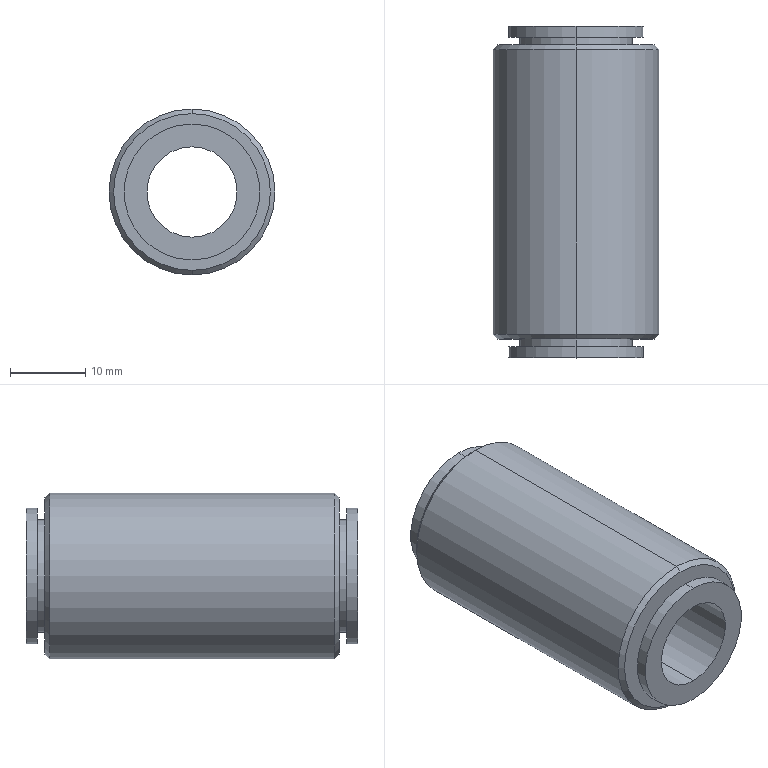Part | STEP file | 1_4 | 1 solid | 22 faces | box 22 x 44 x 22 mm | volume 10940 mm3 | cylinder 12 | plane 6 | cone 4 | commonest cylinder face diameters 15 x4 18 x4 12 x2 22 x2
STEP:
#1=CARTESIAN_POINT('',(0.,40.886,-11.));
#2=VERTEX_POINT('',#1);
#3=CARTESIAN_POINT('',(0.,40.886,11.));
#4=VERTEX_POINT('',#3);
#5=CARTESIAN_POINT('',(0.,40.886,0.));
#6=DIRECTION('',(0.,-1.,0.));
#7=DIRECTION('',(0.,0.,-1.));
#8=AXIS2_PLACEMENT_3D('',#5,#6,#7);
#9=CIRCLE('',#8,11.);
#10=EDGE_CURVE('',#2,#4,#9,.T.);
#11=ORIENTED_EDGE('',*,*,#10,.T.);
#12=CARTESIAN_POINT('',(0.,3.114,11.));
#13=VERTEX_POINT('',#12);
#14=CARTESIAN_POINT('',(0.,22.,11.));
#15=DIRECTION('',(0.,-1.,0.));
#16=VECTOR('',#15,1000.);
#17=LINE('',#14,#16);
#18=EDGE_CURVE('',#4,#13,#17,.T.);
#19=ORIENTED_EDGE('',*,*,#18,.T.);
#20=CARTESIAN_POINT('',(0.,3.114,-11.));
#21=VERTEX_POINT('',#20);
#22=CARTESIAN_POINT('',(0.,3.114,0.));
#23=DIRECTION('',(0.,1.,0.));
#24=DIRECTION('',(0.,0.,-1.));
#25=AXIS2_PLACEMENT_3D('',#22,#23,#24);
#26=CIRCLE('',#25,11.);
#27=EDGE_CURVE('',#13,#21,#26,.T.);
#28=ORIENTED_EDGE('',*,*,#27,.T.);
#29=CARTESIAN_POINT('',(0.,22.,-11.));
#30=DIRECTION('',(0.,-1.,0.));
#31=VECTOR('',#30,1000.);
#32=LINE('',#29,#31);
#33=EDGE_CURVE('',#2,#21,#32,.T.);
#34=ORIENTED_EDGE('',*,*,#33,.F.);
#35=EDGE_LOOP('',(#11,#19,#28,#34));
#36=FACE_OUTER_BOUND('',#35,.T.);
#37=CARTESIAN_POINT('',(0.,22.,0.));
#38=DIRECTION('',(0.,-1.,0.));
#39=DIRECTION('',(0.,0.,-1.));
#40=AXIS2_PLACEMENT_3D('',#37,#38,#39);
#41=CYLINDRICAL_SURFACE('',#40,11.);
#42=ADVANCED_FACE('',(#36),#41,.T.);
#43=CARTESIAN_POINT('',(0.,41.5,-10.386));
#44=VERTEX_POINT('',#43);
#45=CARTESIAN_POINT('',(0.,41.5,10.386));
#46=VERTEX_POINT('',#45);
#47=CARTESIAN_POINT('',(0.,41.5,0.));
#48=DIRECTION('',(0.,-1.,0.));
#49=DIRECTION('',(0.,0.,-1.));
#50=AXIS2_PLACEMENT_3D('',#47,#48,#49);
#51=CIRCLE('',#50,10.386);
#52=EDGE_CURVE('',#44,#46,#51,.T.);
#53=ORIENTED_EDGE('',*,*,#52,.T.);
#54=CARTESIAN_POINT('',(0.,40.886,11.));
#55=DIRECTION('',(0.,-0.7071,0.7071));
#56=VECTOR('',#55,1000.);
#57=LINE('',#54,#56);
#58=EDGE_CURVE('',#46,#4,#57,.T.);
#59=ORIENTED_EDGE('',*,*,#58,.T.);
#60=ORIENTED_EDGE('',*,*,#10,.F.);
#61=CARTESIAN_POINT('',(0.,40.886,-11.));
#62=DIRECTION('',(0.,-0.7071,-0.7071));
#63=VECTOR('',#62,1000.);
#64=LINE('',#61,#63);
#65=EDGE_CURVE('',#44,#2,#64,.T.);
#66=ORIENTED_EDGE('',*,*,#65,.F.);
#67=EDGE_LOOP('',(#53,#59,#60,#66));
#68=FACE_OUTER_BOUND('',#67,.T.);
#69=CARTESIAN_POINT('',(0.,40.886,0.));
#70=DIRECTION('',(0.,-1.,0.));
#71=DIRECTION('',(0.,0.,-1.));
#72=AXIS2_PLACEMENT_3D('',#69,#70,#71);
#73=CONICAL_SURFACE('',#72,11.,0.7854);
#74=ADVANCED_FACE('',(#68),#73,.T.);
#75=CARTESIAN_POINT('',(0.,2.5,10.386));
#76=VERTEX_POINT('',#75);
#77=CARTESIAN_POINT('',(0.,2.5,-10.386));
#78=VERTEX_POINT('',#77);
#79=CARTESIAN_POINT('',(0.,2.5,0.));
#80=DIRECTION('',(0.,1.,0.));
#81=DIRECTION('',(0.,0.,1.));
#82=AXIS2_PLACEMENT_3D('',#79,#80,#81);
#83=CIRCLE('',#82,10.386);
#84=EDGE_CURVE('',#76,#78,#83,.T.);
#85=ORIENTED_EDGE('',*,*,#84,.T.);
#86=CARTESIAN_POINT('',(0.,3.114,-11.));
#87=DIRECTION('',(0.,0.7071,-0.7071));
#88=VECTOR('',#87,1000.);
#89=LINE('',#86,#88);
#90=EDGE_CURVE('',#78,#21,#89,.T.);
#91=ORIENTED_EDGE('',*,*,#90,.T.);
#92=ORIENTED_EDGE('',*,*,#27,.F.);
#93=CARTESIAN_POINT('',(0.,3.114,11.));
#94=DIRECTION('',(0.,0.7071,0.7071));
#95=VECTOR('',#94,1000.);
#96=LINE('',#93,#95);
#97=EDGE_CURVE('',#76,#13,#96,.T.);
#98=ORIENTED_EDGE('',*,*,#97,.F.);
#99=EDGE_LOOP('',(#85,#91,#92,#98));
#100=FACE_OUTER_BOUND('',#99,.T.);
#101=CARTESIAN_POINT('',(0.,3.114,0.));
#102=DIRECTION('',(0.,1.,0.));
#103=DIRECTION('',(0.,0.,1.));
#104=AXIS2_PLACEMENT_3D('',#101,#102,#103);
#105=CONICAL_SURFACE('',#104,11.,0.7854);
#106=ADVANCED_FACE('',(#100),#105,.T.);
#107=CARTESIAN_POINT('',(0.,42.5,-7.5));
#108=VERTEX_POINT('',#107);
#109=CARTESIAN_POINT('',(0.,42.5,7.5));
#110=VERTEX_POINT('',#109);
#111=CARTESIAN_POINT('',(0.,42.5,0.));
#112=DIRECTION('',(0.,-1.,0.));
#113=DIRECTION('',(0.,0.,-1.));
#114=AXIS2_PLACEMENT_3D('',#111,#112,#113);
#115=CIRCLE('',#114,7.5);
#116=EDGE_CURVE('',#108,#110,#115,.T.);
#117=ORIENTED_EDGE('',*,*,#116,.T.);
#118=CARTESIAN_POINT('',(0.,41.5,7.5));
#119=VERTEX_POINT('',#118);
#120=CARTESIAN_POINT('',(0.,42.,7.5));
#121=DIRECTION('',(0.,-1.,0.));
#122=VECTOR('',#121,1000.);
#123=LINE('',#120,#122);
#124=EDGE_CURVE('',#110,#119,#123,.T.);
#125=ORIENTED_EDGE('',*,*,#124,.T.);
#126=CARTESIAN_POINT('',(0.,41.5,-7.5));
#127=VERTEX_POINT('',#126);
#128=CARTESIAN_POINT('',(0.,41.5,0.));
#129=DIRECTION('',(0.,-1.,0.));
#130=DIRECTION('',(0.,0.,-1.));
#131=AXIS2_PLACEMENT_3D('',#128,#129,#130);
#132=CIRCLE('',#131,7.5);
#133=EDGE_CURVE('',#127,#119,#132,.T.);
#134=ORIENTED_EDGE('',*,*,#133,.F.);
#135=CARTESIAN_POINT('',(0.,42.,-7.5));
#136=DIRECTION('',(0.,-1.,0.));
#137=VECTOR('',#136,1000.);
#138=LINE('',#135,#137);
#139=EDGE_CURVE('',#108,#127,#138,.T.);
#140=ORIENTED_EDGE('',*,*,#139,.F.);
#141=EDGE_LOOP('',(#117,#125,#134,#140));
#142=FACE_OUTER_BOUND('',#141,.T.);
#143=CARTESIAN_POINT('',(0.,42.,0.));
#144=DIRECTION('',(0.,-1.,0.));
#145=DIRECTION('',(0.,0.,-1.));
#146=AXIS2_PLACEMENT_3D('',#143,#144,#145);
#147=CYLINDRICAL_SURFACE('',#146,7.5);
#148=ADVANCED_FACE('',(#142),#147,.T.);
#149=CARTESIAN_POINT('',(0.,2.5,7.5));
#150=VERTEX_POINT('',#149);
#151=CARTESIAN_POINT('',(0.,2.5,-7.5));
#152=VERTEX_POINT('',#151);
#153=CARTESIAN_POINT('',(0.,2.5,0.));
#154=DIRECTION('',(0.,1.,0.));
#155=DIRECTION('',(0.,0.,-1.));
#156=AXIS2_PLACEMENT_3D('',#153,#154,#155);
#157=CIRCLE('',#156,7.5);
#158=EDGE_CURVE('',#150,#152,#157,.T.);
#159=ORIENTED_EDGE('',*,*,#158,.F.);
#160=CARTESIAN_POINT('',(0.,1.5,7.5));
#161=VERTEX_POINT('',#160);
#162=CARTESIAN_POINT('',(0.,2.,7.5));
#163=DIRECTION('',(0.,-1.,0.));
#164=VECTOR('',#163,1000.);
#165=LINE('',#162,#164);
#166=EDGE_CURVE('',#150,#161,#165,.T.);
#167=ORIENTED_EDGE('',*,*,#166,.T.);
#168=CARTESIAN_POINT('',(0.,1.5,-7.5));
#169=VERTEX_POINT('',#168);
#170=CARTESIAN_POINT('',(0.,1.5,0.));
#171=DIRECTION('',(0.,1.,0.));
#172=DIRECTION('',(0.,0.,-1.));
#173=AXIS2_PLACEMENT_3D('',#170,#171,#172);
#174=CIRCLE('',#173,7.5);
#175=EDGE_CURVE('',#161,#169,#174,.T.);
#176=ORIENTED_EDGE('',*,*,#175,.T.);
#177=CARTESIAN_POINT('',(0.,2.,-7.5));
#178=DIRECTION('',(0.,-1.,0.));
#179=VECTOR('',#178,1000.);
#180=LINE('',#177,#179);
#181=EDGE_CURVE('',#152,#169,#180,.T.);
#182=ORIENTED_EDGE('',*,*,#181,.F.);
#183=EDGE_LOOP('',(#159,#167,#176,#182));
#184=FACE_OUTER_BOUND('',#183,.T.);
#185=CARTESIAN_POINT('',(0.,2.,0.));
#186=DIRECTION('',(0.,-1.,0.));
#187=DIRECTION('',(0.,0.,-1.));
#188=AXIS2_PLACEMENT_3D('',#185,#186,#187);
#189=CYLINDRICAL_SURFACE('',#188,7.5);
#190=ADVANCED_FACE('',(#184),#189,.T.);
#191=CARTESIAN_POINT('',(0.,44.,-9.));
#192=VERTEX_POINT('',#191);
#193=CARTESIAN_POINT('',(0.,44.,9.));
#194=VERTEX_POINT('',#193);
#195=CARTESIAN_POINT('',(0.,44.,0.));
#196=DIRECTION('',(0.,-1.,0.));
#197=DIRECTION('',(0.,0.,-1.));
#198=AXIS2_PLACEMENT_3D('',#195,#196,#197);
#199=CIRCLE('',#198,9.);
#200=EDGE_CURVE('',#192,#194,#199,.T.);
#201=ORIENTED_EDGE('',*,*,#200,.T.);
#202=CARTESIAN_POINT('',(0.,42.5,9.));
#203=VERTEX_POINT('',#202);
#204=CARTESIAN_POINT('',(0.,43.25,9.));
#205=DIRECTION('',(0.,-1.,0.));
#206=VECTOR('',#205,1000.);
#207=LINE('',#204,#206);
#208=EDGE_CURVE('',#194,#203,#207,.T.);
#209=ORIENTED_EDGE('',*,*,#208,.T.);
#210=CARTESIAN_POINT('',(0.,42.5,-9.));
#211=VERTEX_POINT('',#210);
#212=CARTESIAN_POINT('',(0.,42.5,0.));
#213=DIRECTION('',(0.,-1.,0.));
#214=DIRECTION('',(0.,0.,-1.));
#215=AXIS2_PLACEMENT_3D('',#212,#213,#214);
#216=CIRCLE('',#215,9.);
#217=EDGE_CURVE('',#211,#203,#216,.T.);
#218=ORIENTED_EDGE('',*,*,#217,.F.);
#219=CARTESIAN_POINT('',(0.,43.25,-9.));
#220=DIRECTION('',(0.,-1.,0.));
#221=VECTOR('',#220,1000.);
#222=LINE('',#219,#221);
#223=EDGE_CURVE('',#192,#211,#222,.T.);
#224=ORIENTED_EDGE('',*,*,#223,.F.);
#225=EDGE_LOOP('',(#201,#209,#218,#224));
#226=FACE_OUTER_BOUND('',#225,.T.);
#227=CARTESIAN_POINT('',(0.,43.25,0.));
#228=DIRECTION('',(0.,-1.,0.));
#229=DIRECTION('',(0.,0.,-1.));
#230=AXIS2_PLACEMENT_3D('',#227,#228,#229);
#231=CYLINDRICAL_SURFACE('',#230,9.);
#232=ADVANCED_FACE('',(#226),#231,.T.);
#233=CARTESIAN_POINT('',(0.,1.5,9.));
#234=VERTEX_POINT('',#233);
#235=CARTESIAN_POINT('',(0.,1.5,-9.));
#236=VERTEX_POINT('',#235);
#237=CARTESIAN_POINT('',(0.,1.5,0.));
#238=DIRECTION('',(0.,1.,0.));
#239=DIRECTION('',(0.,0.,-1.));
#240=AXIS2_PLACEMENT_3D('',#237,#238,#239);
#241=CIRCLE('',#240,9.);
#242=EDGE_CURVE('',#234,#236,#241,.T.);
#243=ORIENTED_EDGE('',*,*,#242,.F.);
#244=CARTESIAN_POINT('',(0.,0.,9.));
#245=VERTEX_POINT('',#244);
#246=CARTESIAN_POINT('',(0.,0.75,9.));
#247=DIRECTION('',(0.,-1.,0.));
#248=VECTOR('',#247,1000.);
#249=LINE('',#246,#248);
#250=EDGE_CURVE('',#234,#245,#249,.T.);
#251=ORIENTED_EDGE('',*,*,#250,.T.);
#252=CARTESIAN_POINT('',(0.,0.,-9.));
#253=VERTEX_POINT('',#252);
#254=CARTESIAN_POINT('',(0.,0.,0.));
#255=DIRECTION('',(0.,1.,0.));
#256=DIRECTION('',(0.,0.,-1.));
#257=AXIS2_PLACEMENT_3D('',#254,#255,#256);
#258=CIRCLE('',#257,9.);
#259=EDGE_CURVE('',#245,#253,#258,.T.);
#260=ORIENTED_EDGE('',*,*,#259,.T.);
#261=CARTESIAN_POINT('',(0.,0.75,-9.));
#262=DIRECTION('',(0.,-1.,0.));
#263=VECTOR('',#262,1000.);
#264=LINE('',#261,#263);
#265=EDGE_CURVE('',#236,#253,#264,.T.);
#266=ORIENTED_EDGE('',*,*,#265,.F.);
#267=EDGE_LOOP('',(#243,#251,#260,#266));
#268=FACE_OUTER_BOUND('',#267,.T.);
#269=CARTESIAN_POINT('',(0.,0.75,0.));
#270=DIRECTION('',(0.,-1.,0.));
#271=DIRECTION('',(0.,0.,-1.));
#272=AXIS2_PLACEMENT_3D('',#269,#270,#271);
#273=CYLINDRICAL_SURFACE('',#272,9.);
#274=ADVANCED_FACE('',(#268),#273,.T.);
#275=CARTESIAN_POINT('',(0.,0.,-6.));
#276=VERTEX_POINT('',#275);
#277=CARTESIAN_POINT('',(0.,0.,6.));
#278=VERTEX_POINT('',#277);
#279=CARTESIAN_POINT('',(0.,0.,0.));
#280=DIRECTION('',(0.,1.,0.));
#281=DIRECTION('',(0.,0.,1.));
#282=AXIS2_PLACEMENT_3D('',#279,#280,#281);
#283=CIRCLE('',#282,6.);
#284=EDGE_CURVE('',#276,#278,#283,.T.);
#285=ORIENTED_EDGE('',*,*,#284,.F.);
#286=CARTESIAN_POINT('',(0.,44.,-6.));
#287=VERTEX_POINT('',#286);
#288=CARTESIAN_POINT('',(0.,44.,-6.));
#289=DIRECTION('',(0.,1.,0.));
#290=VECTOR('',#289,1000.);
#291=LINE('',#288,#290);
#292=EDGE_CURVE('',#276,#287,#291,.T.);
#293=ORIENTED_EDGE('',*,*,#292,.T.);
#294=CARTESIAN_POINT('',(0.,44.,6.));
#295=VERTEX_POINT('',#294);
#296=CARTESIAN_POINT('',(0.,44.,0.));
#297=DIRECTION('',(0.,-1.,0.));
#298=DIRECTION('',(0.,0.,1.));
#299=AXIS2_PLACEMENT_3D('',#296,#297,#298);
#300=CIRCLE('',#299,6.);
#301=EDGE_CURVE('',#295,#287,#300,.T.);
#302=ORIENTED_EDGE('',*,*,#301,.F.);
#303=CARTESIAN_POINT('',(0.,44.,6.));
#304=DIRECTION('',(0.,1.,0.));
#305=VECTOR('',#304,1000.);
#306=LINE('',#303,#305);
#307=EDGE_CURVE('',#278,#295,#306,.T.);
#308=ORIENTED_EDGE('',*,*,#307,.F.);
#309=EDGE_LOOP('',(#285,#293,#302,#308));
#310=FACE_OUTER_BOUND('',#309,.T.);
#311=CARTESIAN_POINT('',(0.,44.,0.));
#312=DIRECTION('',(0.,1.,0.));
#313=DIRECTION('',(0.,0.,1.));
#314=AXIS2_PLACEMENT_3D('',#311,#312,#313);
#315=CYLINDRICAL_SURFACE('',#314,6.);
#316=ADVANCED_FACE('',(#310),#315,.F.);
#317=ORIENTED_EDGE('',*,*,#18,.F.);
#318=CARTESIAN_POINT('',(0.,40.886,0.));
#319=DIRECTION('',(0.,-1.,0.));
#320=DIRECTION('',(0.,0.,-1.));
#321=AXIS2_PLACEMENT_3D('',#318,#319,#320);
#322=CIRCLE('',#321,11.);
#323=EDGE_CURVE('',#4,#2,#322,.T.);
#324=ORIENTED_EDGE('',*,*,#323,.T.);
#325=ORIENTED_EDGE('',*,*,#33,.T.);
#326=CARTESIAN_POINT('',(0.,3.114,0.));
#327=DIRECTION('',(0.,1.,0.));
#328=DIRECTION('',(0.,0.,-1.));
#329=AXIS2_PLACEMENT_3D('',#326,#327,#328);
#330=CIRCLE('',#329,11.);
#331=EDGE_CURVE('',#21,#13,#330,.T.);
#332=ORIENTED_EDGE('',*,*,#331,.T.);
#333=EDGE_LOOP('',(#317,#324,#325,#332));
#334=FACE_OUTER_BOUND('',#333,.T.);
#335=CARTESIAN_POINT('',(0.,22.,0.));
#336=DIRECTION('',(0.,-1.,0.));
#337=DIRECTION('',(0.,0.,-1.));
#338=AXIS2_PLACEMENT_3D('',#335,#336,#337);
#339=CYLINDRICAL_SURFACE('',#338,11.);
#340=ADVANCED_FACE('',(#334),#339,.T.);
#341=ORIENTED_EDGE('',*,*,#58,.F.);
#342=CARTESIAN_POINT('',(0.,41.5,0.));
#343=DIRECTION('',(0.,-1.,0.));
#344=DIRECTION('',(0.,0.,-1.));
#345=AXIS2_PLACEMENT_3D('',#342,#343,#344);
#346=CIRCLE('',#345,10.386);
#347=EDGE_CURVE('',#46,#44,#346,.T.);
#348=ORIENTED_EDGE('',*,*,#347,.T.);
#349=ORIENTED_EDGE('',*,*,#65,.T.);
#350=ORIENTED_EDGE('',*,*,#323,.F.);
#351=EDGE_LOOP('',(#341,#348,#349,#350));
#352=FACE_OUTER_BOUND('',#351,.T.);
#353=CARTESIAN_POINT('',(0.,40.886,0.));
#354=DIRECTION('',(0.,-1.,0.));
#355=DIRECTION('',(0.,0.,-1.));
#356=AXIS2_PLACEMENT_3D('',#353,#354,#355);
#357=CONICAL_SURFACE('',#356,11.,0.7854);
#358=ADVANCED_FACE('',(#352),#357,.T.);
#359=ORIENTED_EDGE('',*,*,#90,.F.);
#360=CARTESIAN_POINT('',(0.,2.5,0.));
#361=DIRECTION('',(0.,1.,0.));
#362=DIRECTION('',(0.,0.,1.));
#363=AXIS2_PLACEMENT_3D('',#360,#361,#362);
#364=CIRCLE('',#363,10.386);
#365=EDGE_CURVE('',#78,#76,#364,.T.);
#366=ORIENTED_EDGE('',*,*,#365,.T.);
#367=ORIENTED_EDGE('',*,*,#97,.T.);
#368=ORIENTED_EDGE('',*,*,#331,.F.);
#369=EDGE_LOOP('',(#359,#366,#367,#368));
#370=FACE_OUTER_BOUND('',#369,.T.);
#371=CARTESIAN_POINT('',(0.,3.114,0.));
#372=DIRECTION('',(0.,1.,0.));
#373=DIRECTION('',(0.,0.,1.));
#374=AXIS2_PLACEMENT_3D('',#371,#372,#373);
#375=CONICAL_SURFACE('',#374,11.,0.7854);
#376=ADVANCED_FACE('',(#370),#375,.T.);
#377=ORIENTED_EDGE('',*,*,#52,.F.);
#378=ORIENTED_EDGE('',*,*,#347,.F.);
#379=EDGE_LOOP('',(#377,#378));
#380=FACE_OUTER_BOUND('',#379,.T.);
#381=ORIENTED_EDGE('',*,*,#133,.T.);
#382=CARTESIAN_POINT('',(0.,41.5,0.));
#383=DIRECTION('',(0.,-1.,0.));
#384=DIRECTION('',(0.,0.,-1.));
#385=AXIS2_PLACEMENT_3D('',#382,#383,#384);
#386=CIRCLE('',#385,7.5);
#387=EDGE_CURVE('',#119,#127,#386,.T.);
#388=ORIENTED_EDGE('',*,*,#387,.T.);
#389=EDGE_LOOP('',(#381,#388));
#390=FACE_BOUND('',#389,.T.);
#391=CARTESIAN_POINT('',(8.943,41.5,0.));
#392=DIRECTION('',(0.,1.,0.));
#393=DIRECTION('',(0.,0.,1.));
#394=AXIS2_PLACEMENT_3D('',#391,#392,#393);
#395=PLANE('',#394);
#396=ADVANCED_FACE('',(#380,#390),#395,.T.);
#397=CARTESIAN_POINT('',(0.,2.5,0.));
#398=DIRECTION('',(0.,1.,0.));
#399=DIRECTION('',(0.,0.,-1.));
#400=AXIS2_PLACEMENT_3D('',#397,#398,#399);
#401=CIRCLE('',#400,7.5);
#402=EDGE_CURVE('',#152,#150,#401,.T.);
#403=ORIENTED_EDGE('',*,*,#402,.T.);
#404=ORIENTED_EDGE('',*,*,#158,.T.);
#405=EDGE_LOOP('',(#403,#404));
#406=FACE_BOUND('',#405,.T.);
#407=ORIENTED_EDGE('',*,*,#84,.F.);
#408=ORIENTED_EDGE('',*,*,#365,.F.);
#409=EDGE_LOOP('',(#407,#408));
#410=FACE_OUTER_BOUND('',#409,.T.);
#411=CARTESIAN_POINT('',(8.943,2.5,0.));
#412=DIRECTION('',(0.,-1.,0.));
#413=DIRECTION('',(0.,0.,-1.));
#414=AXIS2_PLACEMENT_3D('',#411,#412,#413);
#415=PLANE('',#414);
#416=ADVANCED_FACE('',(#406,#410),#415,.T.);
#417=ORIENTED_EDGE('',*,*,#124,.F.);
#418=CARTESIAN_POINT('',(0.,42.5,0.));
#419=DIRECTION('',(0.,-1.,0.));
#420=DIRECTION('',(0.,0.,-1.));
#421=AXIS2_PLACEMENT_3D('',#418,#419,#420);
#422=CIRCLE('',#421,7.5);
#423=EDGE_CURVE('',#110,#108,#422,.T.);
#424=ORIENTED_EDGE('',*,*,#423,.T.);
#425=ORIENTED_EDGE('',*,*,#139,.T.);
#426=ORIENTED_EDGE('',*,*,#387,.F.);
#427=EDGE_LOOP('',(#417,#424,#425,#426));
#428=FACE_OUTER_BOUND('',#427,.T.);
#429=CARTESIAN_POINT('',(0.,42.,0.));
#430=DIRECTION('',(0.,-1.,0.));
#431=DIRECTION('',(0.,0.,-1.));
#432=AXIS2_PLACEMENT_3D('',#429,#430,#431);
#433=CYLINDRICAL_SURFACE('',#432,7.5);
#434=ADVANCED_FACE('',(#428),#433,.T.);
#435=ORIENTED_EDGE('',*,*,#166,.F.);
#436=ORIENTED_EDGE('',*,*,#402,.F.);
#437=ORIENTED_EDGE('',*,*,#181,.T.);
#438=CARTESIAN_POINT('',(0.,1.5,0.));
#439=DIRECTION('',(0.,1.,0.));
#440=DIRECTION('',(0.,0.,-1.));
#441=AXIS2_PLACEMENT_3D('',#438,#439,#440);
#442=CIRCLE('',#441,7.5);
#443=EDGE_CURVE('',#169,#161,#442,.T.);
#444=ORIENTED_EDGE('',*,*,#443,.T.);
#445=EDGE_LOOP('',(#435,#436,#437,#444));
#446=FACE_OUTER_BOUND('',#445,.T.);
#447=CARTESIAN_POINT('',(0.,2.,0.));
#448=DIRECTION('',(0.,-1.,0.));
#449=DIRECTION('',(0.,0.,-1.));
#450=AXIS2_PLACEMENT_3D('',#447,#448,#449);
#451=CYLINDRICAL_SURFACE('',#450,7.5);
#452=ADVANCED_FACE('',(#446),#451,.T.);
#453=ORIENTED_EDGE('',*,*,#116,.F.);
#454=ORIENTED_EDGE('',*,*,#423,.F.);
#455=EDGE_LOOP('',(#453,#454));
#456=FACE_BOUND('',#455,.T.);
#457=ORIENTED_EDGE('',*,*,#217,.T.);
#458=CARTESIAN_POINT('',(0.,42.5,0.));
#459=DIRECTION('',(0.,-1.,0.));
#460=DIRECTION('',(0.,0.,-1.));
#461=AXIS2_PLACEMENT_3D('',#458,#459,#460);
#462=CIRCLE('',#461,9.);
#463=EDGE_CURVE('',#203,#211,#462,.T.);
#464=ORIENTED_EDGE('',*,*,#463,.T.);
#465=EDGE_LOOP('',(#457,#464));
#466=FACE_OUTER_BOUND('',#465,.T.);
#467=CARTESIAN_POINT('',(8.25,42.5,0.));
#468=DIRECTION('',(0.,-1.,0.));
#469=DIRECTION('',(0.,0.,-1.));
#470=AXIS2_PLACEMENT_3D('',#467,#468,#469);
#471=PLANE('',#470);
#472=ADVANCED_FACE('',(#456,#466),#471,.T.);
#473=CARTESIAN_POINT('',(0.,1.5,0.));
#474=DIRECTION('',(0.,1.,0.));
#475=DIRECTION('',(0.,0.,-1.));
#476=AXIS2_PLACEMENT_3D('',#473,#474,#475);
#477=CIRCLE('',#476,9.);
#478=EDGE_CURVE('',#236,#234,#477,.T.);
#479=ORIENTED_EDGE('',*,*,#478,.T.);
#480=ORIENTED_EDGE('',*,*,#242,.T.);
#481=EDGE_LOOP('',(#479,#480));
#482=FACE_OUTER_BOUND('',#481,.T.);
#483=ORIENTED_EDGE('',*,*,#443,.F.);
#484=ORIENTED_EDGE('',*,*,#175,.F.);
#485=EDGE_LOOP('',(#483,#484));
#486=FACE_BOUND('',#485,.T.);
#487=CARTESIAN_POINT('',(8.25,1.5,0.));
#488=DIRECTION('',(0.,1.,0.));
#489=DIRECTION('',(0.,0.,1.));
#490=AXIS2_PLACEMENT_3D('',#487,#488,#489);
#491=PLANE('',#490);
#492=ADVANCED_FACE('',(#482,#486),#491,.T.);
#493=ORIENTED_EDGE('',*,*,#208,.F.);
#494=CARTESIAN_POINT('',(0.,44.,0.));
#495=DIRECTION('',(0.,-1.,0.));
#496=DIRECTION('',(0.,0.,-1.));
#497=AXIS2_PLACEMENT_3D('',#494,#495,#496);
#498=CIRCLE('',#497,9.);
#499=EDGE_CURVE('',#194,#192,#498,.T.);
#500=ORIENTED_EDGE('',*,*,#499,.T.);
#501=ORIENTED_EDGE('',*,*,#223,.T.);
#502=ORIENTED_EDGE('',*,*,#463,.F.);
#503=EDGE_LOOP('',(#493,#500,#501,#502));
#504=FACE_OUTER_BOUND('',#503,.T.);
#505=CARTESIAN_POINT('',(0.,43.25,0.));
#506=DIRECTION('',(0.,-1.,0.));
#507=DIRECTION('',(0.,0.,-1.));
#508=AXIS2_PLACEMENT_3D('',#505,#506,#507);
#509=CYLINDRICAL_SURFACE('',#508,9.);
#510=ADVANCED_FACE('',(#504),#509,.T.);
#511=ORIENTED_EDGE('',*,*,#250,.F.);
#512=ORIENTED_EDGE('',*,*,#478,.F.);
#513=ORIENTED_EDGE('',*,*,#265,.T.);
#514=CARTESIAN_POINT('',(0.,0.,0.));
#515=DIRECTION('',(0.,1.,0.));
#516=DIRECTION('',(0.,0.,-1.));
#517=AXIS2_PLACEMENT_3D('',#514,#515,#516);
#518=CIRCLE('',#517,9.);
#519=EDGE_CURVE('',#253,#245,#518,.T.);
#520=ORIENTED_EDGE('',*,*,#519,.T.);
#521=EDGE_LOOP('',(#511,#512,#513,#520));
#522=FACE_OUTER_BOUND('',#521,.T.);
#523=CARTESIAN_POINT('',(0.,0.75,0.));
#524=DIRECTION('',(0.,-1.,0.));
#525=DIRECTION('',(0.,0.,-1.));
#526=AXIS2_PLACEMENT_3D('',#523,#524,#525);
#527=CYLINDRICAL_SURFACE('',#526,9.);
#528=ADVANCED_FACE('',(#522),#527,.T.);
#529=ORIENTED_EDGE('',*,*,#200,.F.);
#530=ORIENTED_EDGE('',*,*,#499,.F.);
#531=EDGE_LOOP('',(#529,#530));
#532=FACE_OUTER_BOUND('',#531,.T.);
#533=ORIENTED_EDGE('',*,*,#301,.T.);
#534=CARTESIAN_POINT('',(0.,44.,0.));
#535=DIRECTION('',(0.,-1.,0.));
#536=DIRECTION('',(0.,0.,1.));
#537=AXIS2_PLACEMENT_3D('',#534,#535,#536);
#538=CIRCLE('',#537,6.);
#539=EDGE_CURVE('',#287,#295,#538,.T.);
#540=ORIENTED_EDGE('',*,*,#539,.T.);
#541=EDGE_LOOP('',(#533,#540));
#542=FACE_BOUND('',#541,.T.);
#543=CARTESIAN_POINT('',(4.5,44.,0.));
#544=DIRECTION('',(0.,1.,0.));
#545=DIRECTION('',(0.,0.,1.));
#546=AXIS2_PLACEMENT_3D('',#543,#544,#545);
#547=PLANE('',#546);
#548=ADVANCED_FACE('',(#532,#542),#547,.T.);
#549=ORIENTED_EDGE('',*,*,#519,.F.);
#550=ORIENTED_EDGE('',*,*,#259,.F.);
#551=EDGE_LOOP('',(#549,#550));
#552=FACE_OUTER_BOUND('',#551,.T.);
#553=CARTESIAN_POINT('',(0.,0.,0.));
#554=DIRECTION('',(0.,1.,0.));
#555=DIRECTION('',(0.,0.,1.));
#556=AXIS2_PLACEMENT_3D('',#553,#554,#555);
#557=CIRCLE('',#556,6.);
#558=EDGE_CURVE('',#278,#276,#557,.T.);
#559=ORIENTED_EDGE('',*,*,#558,.T.);
#560=ORIENTED_EDGE('',*,*,#284,.T.);
#561=EDGE_LOOP('',(#559,#560));
#562=FACE_BOUND('',#561,.T.);
#563=CARTESIAN_POINT('',(4.5,0.,0.));
#564=DIRECTION('',(0.,-1.,0.));
#565=DIRECTION('',(0.,0.,-1.));
#566=AXIS2_PLACEMENT_3D('',#563,#564,#565);
#567=PLANE('',#566);
#568=ADVANCED_FACE('',(#552,#562),#567,.T.);
#569=ORIENTED_EDGE('',*,*,#292,.F.);
#570=ORIENTED_EDGE('',*,*,#558,.F.);
#571=ORIENTED_EDGE('',*,*,#307,.T.);
#572=ORIENTED_EDGE('',*,*,#539,.F.);
#573=EDGE_LOOP('',(#569,#570,#571,#572));
#574=FACE_OUTER_BOUND('',#573,.T.);
#575=CARTESIAN_POINT('',(0.,44.,0.));
#576=DIRECTION('',(0.,1.,0.));
#577=DIRECTION('',(0.,0.,1.));
#578=AXIS2_PLACEMENT_3D('',#575,#576,#577);
#579=CYLINDRICAL_SURFACE('',#578,6.);
#580=ADVANCED_FACE('',(#574),#579,.F.);
#581=CLOSED_SHELL('',(#42,#74,#106,#148,#190,#232,#274,#316,#340,#358,#376,#396,#416,#434,#452,#472,#492,#510,#528,#548,#568,#580));
#582=MANIFOLD_SOLID_BREP('',#581);
#583=CARTESIAN_POINT('',(0.,0.,0.));
#584=DIRECTION('',(0.,0.,1.));
#585=DIRECTION('',(1.,0.,0.));
#586=AXIS2_PLACEMENT_3D('',#583,#584,#585);
#587=(LENGTH_UNIT()NAMED_UNIT(*)SI_UNIT(.MILLI.,.METRE.));
#588=UNCERTAINTY_MEASURE_WITH_UNIT(LENGTH_MEASURE(0.00001),#587,'','');
#589=(NAMED_UNIT(*)PLANE_ANGLE_UNIT()SI_UNIT($,.RADIAN.));
#590=(NAMED_UNIT(*)SI_UNIT($,.STERADIAN.)SOLID_ANGLE_UNIT());
#591=(GEOMETRIC_REPRESENTATION_CONTEXT(3)GLOBAL_UNCERTAINTY_ASSIGNED_CONTEXT((#588))GLOBAL_UNIT_ASSIGNED_CONTEXT((#587,#589,#590))REPRESENTATION_CONTEXT('',''));
#592=ADVANCED_BREP_SHAPE_REPRESENTATION('',(#582,#586),#591);